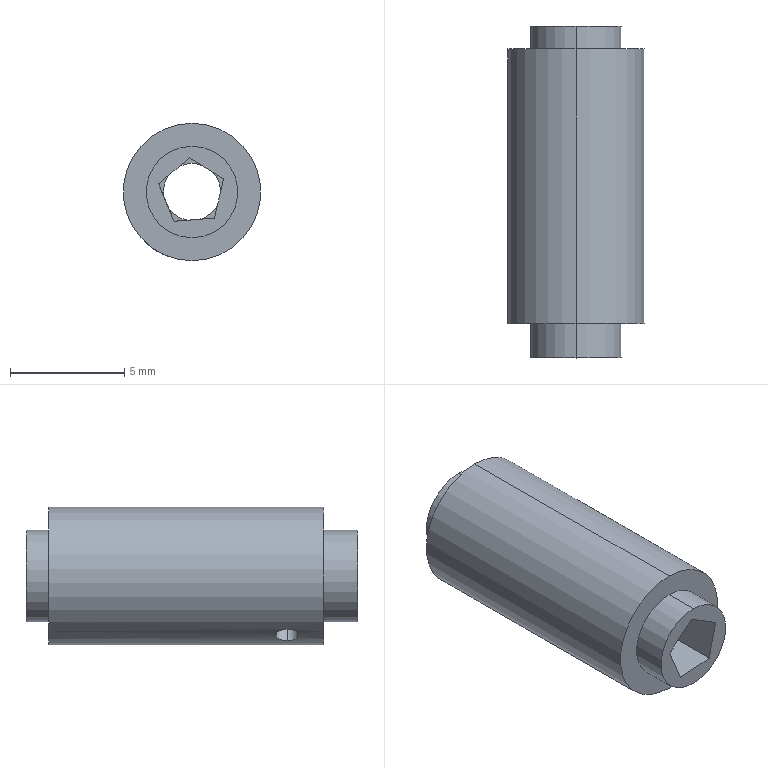Part | SolidWorks | features ICE 6, Extrusion 1 | 1 solid | 27 faces | box 6 x 14.5 x 6 mm | volume 290.19 mm3 | plane 15 | cylinder 12 | commonest cylinder face diameters 4 x4 1 x2 2.5 x2 3 x2 6 x2
STEP:
#1=CARTESIAN_POINT('',(-1.9,1.589,-2.322));
#2=VERTEX_POINT('',#1);
#3=CARTESIAN_POINT('',(-1.031,1.589,-2.817));
#4=VERTEX_POINT('',#3);
#5=CARTESIAN_POINT('',(-1.9,1.589,-2.322));
#6=CARTESIAN_POINT('',(-1.9,1.459,-2.322));
#7=CARTESIAN_POINT('',(-1.858,1.328,-2.357));
#8=CARTESIAN_POINT('',(-1.709,1.143,-2.467));
#9=CARTESIAN_POINT('',(-1.602,1.089,-2.54));
#10=CARTESIAN_POINT('',(-1.372,1.089,-2.671));
#11=CARTESIAN_POINT('',(-1.255,1.144,-2.727));
#12=CARTESIAN_POINT('',(-1.084,1.328,-2.799));
#13=CARTESIAN_POINT('',(-1.031,1.457,-2.817));
#14=CARTESIAN_POINT('',(-1.031,1.589,-2.817));
#15=B_SPLINE_CURVE_WITH_KNOTS('',3,(#5,#6,#7,#8,#9,#10,#11,#12,#13,#14),.UNSPECIFIED.,.F.,.F.,(4,2,2,2,4),(0.001566,0.001958,0.002349,0.002741,0.003132),.UNSPECIFIED.);
#16=EDGE_CURVE('',#2,#4,#15,.T.);
#17=ORIENTED_EDGE('',*,*,#16,.F.);
#18=CARTESIAN_POINT('',(-0.9761,1.589,-0.8146));
#19=VERTEX_POINT('',#18);
#20=CARTESIAN_POINT('',(-2.503,1.589,-3.306));
#21=DIRECTION('',(0.5226,0.,0.8526));
#22=VECTOR('',#21,1000.);
#23=LINE('',#20,#22);
#24=EDGE_CURVE('',#2,#19,#23,.T.);
#25=ORIENTED_EDGE('',*,*,#24,.T.);
#26=CARTESIAN_POINT('',(-0.7839,1.098,-1.279));
#27=VERTEX_POINT('',#26);
#28=CARTESIAN_POINT('',(-0.9761,1.589,-0.8146));
#29=CARTESIAN_POINT('',(-0.9761,1.338,-0.8146));
#30=CARTESIAN_POINT('',(-0.9005,1.145,-0.9973));
#31=CARTESIAN_POINT('',(-0.7839,1.098,-1.279));
#32=(BOUNDED_CURVE()B_SPLINE_CURVE(3,(#28,#29,#30,#31),.UNSPECIFIED.,.F.,.F.)B_SPLINE_CURVE_WITH_KNOTS((4,4),(3.142,4.524),.UNSPECIFIED.)CURVE()GEOMETRIC_REPRESENTATION_ITEM()RATIONAL_B_SPLINE_CURVE((1.,0.8469,0.8469,1.))REPRESENTATION_ITEM(''));
#33=EDGE_CURVE('',#19,#27,#32,.T.);
#34=ORIENTED_EDGE('',*,*,#33,.T.);
#35=CARTESIAN_POINT('',(-0.05259,1.589,-1.221));
#36=VERTEX_POINT('',#35);
#37=CARTESIAN_POINT('',(-0.7839,1.098,-1.279));
#38=CARTESIAN_POINT('',(-0.374,1.035,-1.247));
#39=CARTESIAN_POINT('',(-0.05259,1.251,-1.221));
#40=CARTESIAN_POINT('',(-0.05259,1.589,-1.221));
#41=(BOUNDED_CURVE()B_SPLINE_CURVE(3,(#37,#38,#39,#40),.UNSPECIFIED.,.F.,.F.)B_SPLINE_CURVE_WITH_KNOTS((4,4),(1.383,3.142),.UNSPECIFIED.)CURVE()GEOMETRIC_REPRESENTATION_ITEM()RATIONAL_B_SPLINE_CURVE((1.,0.7584,0.7584,1.))REPRESENTATION_ITEM(''));
#42=EDGE_CURVE('',#27,#36,#41,.T.);
#43=ORIENTED_EDGE('',*,*,#42,.T.);
#44=CARTESIAN_POINT('',(-1.651,1.589,-3.829));
#45=DIRECTION('',(0.5226,0.,0.8526));
#46=VECTOR('',#45,1000.);
#47=LINE('',#44,#46);
#48=EDGE_CURVE('',#4,#36,#47,.T.);
#49=ORIENTED_EDGE('',*,*,#48,.F.);
#50=EDGE_LOOP('',(#17,#25,#34,#43,#49));
#51=FACE_OUTER_BOUND('',#50,.T.);
#52=CARTESIAN_POINT('',(-2.077,1.589,-3.567));
#53=DIRECTION('',(0.5226,0.,0.8526));
#54=DIRECTION('',(0.8526,0.,-0.5226));
#55=AXIS2_PLACEMENT_3D('',#52,#53,#54);
#56=CYLINDRICAL_SURFACE('',#55,0.5);
#57=ADVANCED_FACE('',(#51),#56,.F.);
#58=CARTESIAN_POINT('',(0.,4.5,-1.5));
#59=VERTEX_POINT('',#58);
#60=CARTESIAN_POINT('',(-0.7839,4.5,-1.279));
#61=VERTEX_POINT('',#60);
#62=CARTESIAN_POINT('',(0.,4.5,0.));
#63=DIRECTION('',(0.,1.,0.));
#64=DIRECTION('',(0.,0.,1.));
#65=AXIS2_PLACEMENT_3D('',#62,#63,#64);
#66=CIRCLE('',#65,1.5);
#67=EDGE_CURVE('',#59,#61,#66,.T.);
#68=ORIENTED_EDGE('',*,*,#67,.F.);
#69=CARTESIAN_POINT('',(0.,7.,-1.5));
#70=VERTEX_POINT('',#69);
#71=CARTESIAN_POINT('',(0.,4.5,-1.5));
#72=DIRECTION('',(0.,1.,0.));
#73=VECTOR('',#72,1000.);
#74=LINE('',#71,#73);
#75=EDGE_CURVE('',#59,#70,#74,.T.);
#76=ORIENTED_EDGE('',*,*,#75,.T.);
#77=CARTESIAN_POINT('',(0.,7.,1.5));
#78=VERTEX_POINT('',#77);
#79=CARTESIAN_POINT('',(0.,7.,0.));
#80=DIRECTION('',(0.,1.,0.));
#81=DIRECTION('',(0.,0.,1.));
#82=AXIS2_PLACEMENT_3D('',#79,#80,#81);
#83=CIRCLE('',#82,1.5);
#84=EDGE_CURVE('',#70,#78,#83,.T.);
#85=ORIENTED_EDGE('',*,*,#84,.T.);
#86=CARTESIAN_POINT('',(0.,4.5,1.5));
#87=VERTEX_POINT('',#86);
#88=CARTESIAN_POINT('',(0.,4.5,1.5));
#89=DIRECTION('',(0.,1.,0.));
#90=VECTOR('',#89,1000.);
#91=LINE('',#88,#90);
#92=EDGE_CURVE('',#87,#78,#91,.T.);
#93=ORIENTED_EDGE('',*,*,#92,.F.);
#94=CARTESIAN_POINT('',(-0.1176,4.5,1.495));
#95=VERTEX_POINT('',#94);
#96=CARTESIAN_POINT('',(0.,4.5,0.));
#97=DIRECTION('',(0.,1.,0.));
#98=DIRECTION('',(0.,0.,1.));
#99=AXIS2_PLACEMENT_3D('',#96,#97,#98);
#100=CIRCLE('',#99,1.5);
#101=EDGE_CURVE('',#95,#87,#100,.T.);
#102=ORIENTED_EDGE('',*,*,#101,.F.);
#103=CARTESIAN_POINT('',(-1.459,4.5,0.3503));
#104=VERTEX_POINT('',#103);
#105=CARTESIAN_POINT('',(0.,4.5,0.));
#106=DIRECTION('',(0.,1.,0.));
#107=DIRECTION('',(0.,0.,1.));
#108=AXIS2_PLACEMENT_3D('',#105,#106,#107);
#109=CIRCLE('',#108,1.5);
#110=EDGE_CURVE('',#104,#95,#109,.T.);
#111=ORIENTED_EDGE('',*,*,#110,.F.);
#112=CARTESIAN_POINT('',(0.,4.5,0.));
#113=DIRECTION('',(0.,1.,0.));
#114=DIRECTION('',(0.,0.,1.));
#115=AXIS2_PLACEMENT_3D('',#112,#113,#114);
#116=CIRCLE('',#115,1.5);
#117=EDGE_CURVE('',#61,#104,#116,.T.);
#118=ORIENTED_EDGE('',*,*,#117,.F.);
#119=EDGE_LOOP('',(#68,#76,#85,#93,#102,#111,#118));
#120=FACE_OUTER_BOUND('',#119,.T.);
#121=CARTESIAN_POINT('',(0.,4.5,0.));
#122=DIRECTION('',(0.,1.,0.));
#123=DIRECTION('',(0.,0.,1.));
#124=AXIS2_PLACEMENT_3D('',#121,#122,#123);
#125=CYLINDRICAL_SURFACE('',#124,1.5);
#126=ADVANCED_FACE('',(#120),#125,.F.);
#127=CARTESIAN_POINT('',(0.,7.,-1.25));
#128=VERTEX_POINT('',#127);
#129=CARTESIAN_POINT('',(0.,7.,1.25));
#130=VERTEX_POINT('',#129);
#131=CARTESIAN_POINT('',(0.,7.,0.));
#132=DIRECTION('',(0.,1.,0.));
#133=DIRECTION('',(0.,0.,1.));
#134=AXIS2_PLACEMENT_3D('',#131,#132,#133);
#135=CIRCLE('',#134,1.25);
#136=EDGE_CURVE('',#128,#130,#135,.T.);
#137=ORIENTED_EDGE('',*,*,#136,.F.);
#138=CARTESIAN_POINT('',(0.,13.,-1.25));
#139=VERTEX_POINT('',#138);
#140=CARTESIAN_POINT('',(0.,7.,-1.25));
#141=DIRECTION('',(0.,1.,0.));
#142=VECTOR('',#141,1000.);
#143=LINE('',#140,#142);
#144=EDGE_CURVE('',#128,#139,#143,.T.);
#145=ORIENTED_EDGE('',*,*,#144,.T.);
#146=CARTESIAN_POINT('',(0.,13.,1.25));
#147=VERTEX_POINT('',#146);
#148=CARTESIAN_POINT('',(0.,13.,0.));
#149=DIRECTION('',(0.,1.,0.));
#150=DIRECTION('',(0.,0.,1.));
#151=AXIS2_PLACEMENT_3D('',#148,#149,#150);
#152=CIRCLE('',#151,1.25);
#153=EDGE_CURVE('',#139,#147,#152,.T.);
#154=ORIENTED_EDGE('',*,*,#153,.T.);
#155=CARTESIAN_POINT('',(0.,7.,1.25));
#156=DIRECTION('',(0.,1.,0.));
#157=VECTOR('',#156,1000.);
#158=LINE('',#155,#157);
#159=EDGE_CURVE('',#130,#147,#158,.T.);
#160=ORIENTED_EDGE('',*,*,#159,.F.);
#161=EDGE_LOOP('',(#137,#145,#154,#160));
#162=FACE_OUTER_BOUND('',#161,.T.);
#163=CARTESIAN_POINT('',(0.,7.,0.));
#164=DIRECTION('',(0.,1.,0.));
#165=DIRECTION('',(0.,0.,1.));
#166=AXIS2_PLACEMENT_3D('',#163,#164,#165);
#167=CYLINDRICAL_SURFACE('',#166,1.25);
#168=ADVANCED_FACE('',(#162),#167,.F.);
#169=CARTESIAN_POINT('',(0.,-1.5,-2.));
#170=VERTEX_POINT('',#169);
#171=CARTESIAN_POINT('',(0.,-1.5,2.));
#172=VERTEX_POINT('',#171);
#173=CARTESIAN_POINT('',(0.,-1.5,0.));
#174=DIRECTION('',(0.,-1.,0.));
#175=DIRECTION('',(0.,0.,-1.));
#176=AXIS2_PLACEMENT_3D('',#173,#174,#175);
#177=CIRCLE('',#176,2.);
#178=EDGE_CURVE('',#170,#172,#177,.T.);
#179=ORIENTED_EDGE('',*,*,#178,.F.);
#180=CARTESIAN_POINT('',(0.,0.,-2.));
#181=VERTEX_POINT('',#180);
#182=CARTESIAN_POINT('',(0.,-1.5,-2.));
#183=DIRECTION('',(0.,1.,0.));
#184=VECTOR('',#183,1000.);
#185=LINE('',#182,#184);
#186=EDGE_CURVE('',#170,#181,#185,.T.);
#187=ORIENTED_EDGE('',*,*,#186,.T.);
#188=CARTESIAN_POINT('',(0.,0.,2.));
#189=VERTEX_POINT('',#188);
#190=CARTESIAN_POINT('',(0.,0.,0.));
#191=DIRECTION('',(0.,-1.,0.));
#192=DIRECTION('',(0.,0.,-1.));
#193=AXIS2_PLACEMENT_3D('',#190,#191,#192);
#194=CIRCLE('',#193,2.);
#195=EDGE_CURVE('',#181,#189,#194,.T.);
#196=ORIENTED_EDGE('',*,*,#195,.T.);
#197=CARTESIAN_POINT('',(0.,-1.5,2.));
#198=DIRECTION('',(0.,1.,0.));
#199=VECTOR('',#198,1000.);
#200=LINE('',#197,#199);
#201=EDGE_CURVE('',#172,#189,#200,.T.);
#202=ORIENTED_EDGE('',*,*,#201,.F.);
#203=EDGE_LOOP('',(#179,#187,#196,#202));
#204=FACE_OUTER_BOUND('',#203,.T.);
#205=CARTESIAN_POINT('',(0.,-1.5,0.));
#206=DIRECTION('',(0.,1.,0.));
#207=DIRECTION('',(0.,0.,1.));
#208=AXIS2_PLACEMENT_3D('',#205,#206,#207);
#209=CYLINDRICAL_SURFACE('',#208,2.);
#210=ADVANCED_FACE('',(#204),#209,.T.);
#211=CARTESIAN_POINT('',(0.,13.,2.));
#212=VERTEX_POINT('',#211);
#213=CARTESIAN_POINT('',(0.,13.,-2.));
#214=VERTEX_POINT('',#213);
#215=CARTESIAN_POINT('',(0.,13.,0.));
#216=DIRECTION('',(0.,1.,0.));
#217=DIRECTION('',(0.,0.,1.));
#218=AXIS2_PLACEMENT_3D('',#215,#216,#217);
#219=CIRCLE('',#218,2.);
#220=EDGE_CURVE('',#212,#214,#219,.T.);
#221=ORIENTED_EDGE('',*,*,#220,.F.);
#222=CARTESIAN_POINT('',(0.,12.,2.));
#223=VERTEX_POINT('',#222);
#224=CARTESIAN_POINT('',(0.,13.,2.));
#225=DIRECTION('',(0.,-1.,0.));
#226=VECTOR('',#225,1000.);
#227=LINE('',#224,#226);
#228=EDGE_CURVE('',#212,#223,#227,.T.);
#229=ORIENTED_EDGE('',*,*,#228,.T.);
#230=CARTESIAN_POINT('',(0.,12.,-2.));
#231=VERTEX_POINT('',#230);
#232=CARTESIAN_POINT('',(0.,12.,0.));
#233=DIRECTION('',(0.,1.,0.));
#234=DIRECTION('',(0.,0.,1.));
#235=AXIS2_PLACEMENT_3D('',#232,#233,#234);
#236=CIRCLE('',#235,2.);
#237=EDGE_CURVE('',#223,#231,#236,.T.);
#238=ORIENTED_EDGE('',*,*,#237,.T.);
#239=CARTESIAN_POINT('',(0.,13.,-2.));
#240=DIRECTION('',(0.,-1.,0.));
#241=VECTOR('',#240,1000.);
#242=LINE('',#239,#241);
#243=EDGE_CURVE('',#214,#231,#242,.T.);
#244=ORIENTED_EDGE('',*,*,#243,.F.);
#245=EDGE_LOOP('',(#221,#229,#238,#244));
#246=FACE_OUTER_BOUND('',#245,.T.);
#247=CARTESIAN_POINT('',(0.,13.,0.));
#248=DIRECTION('',(0.,-1.,0.));
#249=DIRECTION('',(0.,0.,-1.));
#250=AXIS2_PLACEMENT_3D('',#247,#248,#249);
#251=CYLINDRICAL_SURFACE('',#250,2.);
#252=ADVANCED_FACE('',(#246),#251,.T.);
#253=CARTESIAN_POINT('',(0.,12.,3.));
#254=VERTEX_POINT('',#253);
#255=CARTESIAN_POINT('',(0.,12.,-3.));
#256=VERTEX_POINT('',#255);
#257=CARTESIAN_POINT('',(0.,12.,0.));
#258=DIRECTION('',(0.,1.,0.));
#259=DIRECTION('',(0.,0.,1.));
#260=AXIS2_PLACEMENT_3D('',#257,#258,#259);
#261=CIRCLE('',#260,3.);
#262=EDGE_CURVE('',#254,#256,#261,.T.);
#263=ORIENTED_EDGE('',*,*,#262,.F.);
#264=CARTESIAN_POINT('',(0.,0.,3.));
#265=VERTEX_POINT('',#264);
#266=CARTESIAN_POINT('',(0.,12.,3.));
#267=DIRECTION('',(0.,-1.,0.));
#268=VECTOR('',#267,1000.);
#269=LINE('',#266,#268);
#270=EDGE_CURVE('',#254,#265,#269,.T.);
#271=ORIENTED_EDGE('',*,*,#270,.T.);
#272=CARTESIAN_POINT('',(0.,0.,-3.));
#273=VERTEX_POINT('',#272);
#274=CARTESIAN_POINT('',(0.,0.,0.));
#275=DIRECTION('',(0.,1.,0.));
#276=DIRECTION('',(0.,0.,1.));
#277=AXIS2_PLACEMENT_3D('',#274,#275,#276);
#278=CIRCLE('',#277,3.);
#279=EDGE_CURVE('',#265,#273,#278,.T.);
#280=ORIENTED_EDGE('',*,*,#279,.T.);
#281=CARTESIAN_POINT('',(0.,12.,-3.));
#282=DIRECTION('',(0.,-1.,0.));
#283=VECTOR('',#282,1000.);
#284=LINE('',#281,#283);
#285=EDGE_CURVE('',#256,#273,#284,.T.);
#286=ORIENTED_EDGE('',*,*,#285,.F.);
#287=EDGE_LOOP('',(#263,#271,#280,#286));
#288=FACE_OUTER_BOUND('',#287,.T.);
#289=CARTESIAN_POINT('',(0.,12.,0.));
#290=DIRECTION('',(0.,-1.,0.));
#291=DIRECTION('',(0.,0.,-1.));
#292=AXIS2_PLACEMENT_3D('',#289,#290,#291);
#293=CYLINDRICAL_SURFACE('',#292,3.);
#294=ADVANCED_FACE('',(#288),#293,.T.);
#295=ORIENTED_EDGE('',*,*,#270,.F.);
#296=CARTESIAN_POINT('',(0.,12.,0.));
#297=DIRECTION('',(0.,1.,0.));
#298=DIRECTION('',(0.,0.,1.));
#299=AXIS2_PLACEMENT_3D('',#296,#297,#298);
#300=CIRCLE('',#299,3.);
#301=EDGE_CURVE('',#256,#254,#300,.T.);
#302=ORIENTED_EDGE('',*,*,#301,.F.);
#303=ORIENTED_EDGE('',*,*,#285,.T.);
#304=CARTESIAN_POINT('',(0.,0.,0.));
#305=DIRECTION('',(0.,1.,0.));
#306=DIRECTION('',(0.,0.,1.));
#307=AXIS2_PLACEMENT_3D('',#304,#305,#306);
#308=CIRCLE('',#307,3.);
#309=EDGE_CURVE('',#273,#265,#308,.T.);
#310=ORIENTED_EDGE('',*,*,#309,.T.);
#311=EDGE_LOOP('',(#295,#302,#303,#310));
#312=FACE_OUTER_BOUND('',#311,.T.);
#313=CARTESIAN_POINT('',(-1.031,1.589,-2.817));
#314=CARTESIAN_POINT('',(-1.031,1.722,-2.817));
#315=CARTESIAN_POINT('',(-1.083,1.851,-2.799));
#316=CARTESIAN_POINT('',(-1.255,2.035,-2.727));
#317=CARTESIAN_POINT('',(-1.373,2.089,-2.671));
#318=CARTESIAN_POINT('',(-1.6,2.09,-2.541));
#319=CARTESIAN_POINT('',(-1.708,2.036,-2.468));
#320=CARTESIAN_POINT('',(-1.859,1.85,-2.357));
#321=CARTESIAN_POINT('',(-1.9,1.72,-2.322));
#322=CARTESIAN_POINT('',(-1.9,1.589,-2.322));
#323=B_SPLINE_CURVE_WITH_KNOTS('',3,(#313,#314,#315,#316,#317,#318,#319,#320,#321,#322),.UNSPECIFIED.,.F.,.F.,(4,2,2,2,4),(0.,0.0003916,0.0007832,0.001175,0.001566),.UNSPECIFIED.);
#324=EDGE_CURVE('',#4,#2,#323,.T.);
#325=ORIENTED_EDGE('',*,*,#324,.T.);
#326=ORIENTED_EDGE('',*,*,#16,.T.);
#327=EDGE_LOOP('',(#325,#326));
#328=FACE_BOUND('',#327,.T.);
#329=CARTESIAN_POINT('',(0.,12.,0.));
#330=DIRECTION('',(0.,-1.,0.));
#331=DIRECTION('',(0.,0.,-1.));
#332=AXIS2_PLACEMENT_3D('',#329,#330,#331);
#333=CYLINDRICAL_SURFACE('',#332,3.);
#334=ADVANCED_FACE('',(#312,#328),#333,.T.);
#335=ORIENTED_EDGE('',*,*,#42,.F.);
#336=CARTESIAN_POINT('',(-0.7839,-1.5,-1.279));
#337=VERTEX_POINT('',#336);
#338=CARTESIAN_POINT('',(-0.7839,4.5,-1.279));
#339=DIRECTION('',(0.,-1.,0.));
#340=VECTOR('',#339,1000.);
#341=LINE('',#338,#340);
#342=EDGE_CURVE('',#27,#337,#341,.T.);
#343=ORIENTED_EDGE('',*,*,#342,.T.);
#344=CARTESIAN_POINT('',(0.9741,-1.5,-1.141));
#345=VERTEX_POINT('',#344);
#346=CARTESIAN_POINT('',(-0.7839,-1.5,-1.279));
#347=DIRECTION('',(0.9969,0.,0.07838));
#348=VECTOR('',#347,1000.);
#349=LINE('',#346,#348);
#350=EDGE_CURVE('',#337,#345,#349,.T.);
#351=ORIENTED_EDGE('',*,*,#350,.T.);
#352=CARTESIAN_POINT('',(0.9741,4.5,-1.141));
#353=VERTEX_POINT('',#352);
#354=CARTESIAN_POINT('',(0.9741,4.5,-1.141));
#355=DIRECTION('',(0.,-1.,0.));
#356=VECTOR('',#355,1000.);
#357=LINE('',#354,#356);
#358=EDGE_CURVE('',#353,#345,#357,.T.);
#359=ORIENTED_EDGE('',*,*,#358,.F.);
#360=CARTESIAN_POINT('',(-0.7839,4.5,-1.279));
#361=DIRECTION('',(0.9969,0.,0.07838));
#362=VECTOR('',#361,1000.);
#363=LINE('',#360,#362);
#364=EDGE_CURVE('',#61,#353,#363,.T.);
#365=ORIENTED_EDGE('',*,*,#364,.F.);
#366=CARTESIAN_POINT('',(-0.7839,2.081,-1.279));
#367=VERTEX_POINT('',#366);
#368=CARTESIAN_POINT('',(-0.7839,4.5,-1.279));
#369=DIRECTION('',(0.,-1.,0.));
#370=VECTOR('',#369,1000.);
#371=LINE('',#368,#370);
#372=EDGE_CURVE('',#61,#367,#371,.T.);
#373=ORIENTED_EDGE('',*,*,#372,.T.);
#374=CARTESIAN_POINT('',(-0.05259,1.589,-1.221));
#375=CARTESIAN_POINT('',(-0.05259,1.928,-1.221));
#376=CARTESIAN_POINT('',(-0.374,2.144,-1.247));
#377=CARTESIAN_POINT('',(-0.7839,2.081,-1.279));
#378=(BOUNDED_CURVE()B_SPLINE_CURVE(3,(#374,#375,#376,#377),.UNSPECIFIED.,.F.,.F.)B_SPLINE_CURVE_WITH_KNOTS((4,4),(3.142,4.9),.UNSPECIFIED.)CURVE()GEOMETRIC_REPRESENTATION_ITEM()RATIONAL_B_SPLINE_CURVE((1.,0.7584,0.7584,1.))REPRESENTATION_ITEM(''));
#379=EDGE_CURVE('',#36,#367,#378,.T.);
#380=ORIENTED_EDGE('',*,*,#379,.F.);
#381=EDGE_LOOP('',(#335,#343,#351,#359,#365,#373,#380));
#382=FACE_OUTER_BOUND('',#381,.T.);
#383=CARTESIAN_POINT('',(-0.7839,4.5,-1.279));
#384=DIRECTION('',(0.07838,0.,-0.9969));
#385=DIRECTION('',(-0.9969,0.,-0.07838));
#386=AXIS2_PLACEMENT_3D('',#383,#384,#385);
#387=PLANE('',#386);
#388=ADVANCED_FACE('',(#382),#387,.F.);
#389=CARTESIAN_POINT('',(-0.7839,2.081,-1.279));
#390=CARTESIAN_POINT('',(-0.9005,2.034,-0.9973));
#391=CARTESIAN_POINT('',(-0.9761,1.84,-0.8146));
#392=CARTESIAN_POINT('',(-0.9761,1.589,-0.8146));
#393=(BOUNDED_CURVE()B_SPLINE_CURVE(3,(#389,#390,#391,#392),.UNSPECIFIED.,.F.,.T.)B_SPLINE_CURVE_WITH_KNOTS((4,4),(1.759,3.142),.UNSPECIFIED.)CURVE()GEOMETRIC_REPRESENTATION_ITEM()RATIONAL_B_SPLINE_CURVE((1.,0.8469,0.8469,1.))REPRESENTATION_ITEM(''));
#394=EDGE_CURVE('',#367,#19,#393,.T.);
#395=ORIENTED_EDGE('',*,*,#394,.F.);
#396=ORIENTED_EDGE('',*,*,#372,.F.);
#397=CARTESIAN_POINT('',(-1.459,4.5,0.3503));
#398=DIRECTION('',(0.3826,0.,-0.9239));
#399=VECTOR('',#398,1000.);
#400=LINE('',#397,#399);
#401=EDGE_CURVE('',#104,#61,#400,.T.);
#402=ORIENTED_EDGE('',*,*,#401,.F.);
#403=CARTESIAN_POINT('',(-1.459,-1.5,0.3503));
#404=VERTEX_POINT('',#403);
#405=CARTESIAN_POINT('',(-1.459,4.5,0.3503));
#406=DIRECTION('',(0.,-1.,0.));
#407=VECTOR('',#406,1000.);
#408=LINE('',#405,#407);
#409=EDGE_CURVE('',#104,#404,#408,.T.);
#410=ORIENTED_EDGE('',*,*,#409,.T.);
#411=CARTESIAN_POINT('',(-1.459,-1.5,0.3503));
#412=DIRECTION('',(0.3826,0.,-0.9239));
#413=VECTOR('',#412,1000.);
#414=LINE('',#411,#413);
#415=EDGE_CURVE('',#404,#337,#414,.T.);
#416=ORIENTED_EDGE('',*,*,#415,.T.);
#417=ORIENTED_EDGE('',*,*,#342,.F.);
#418=ORIENTED_EDGE('',*,*,#33,.F.);
#419=EDGE_LOOP('',(#395,#396,#402,#410,#416,#417,#418));
#420=FACE_OUTER_BOUND('',#419,.T.);
#421=CARTESIAN_POINT('',(-1.459,4.5,0.3503));
#422=DIRECTION('',(-0.9239,0.,-0.3826));
#423=DIRECTION('',(-0.3826,0.,0.9239));
#424=AXIS2_PLACEMENT_3D('',#421,#422,#423);
#425=PLANE('',#424);
#426=ADVANCED_FACE('',(#420),#425,.F.);
#427=CARTESIAN_POINT('',(0.,4.5,0.));
#428=DIRECTION('',(0.,1.,0.));
#429=DIRECTION('',(0.,0.,1.));
#430=AXIS2_PLACEMENT_3D('',#427,#428,#429);
#431=CIRCLE('',#430,1.5);
#432=EDGE_CURVE('',#353,#59,#431,.T.);
#433=ORIENTED_EDGE('',*,*,#432,.T.);
#434=ORIENTED_EDGE('',*,*,#67,.T.);
#435=ORIENTED_EDGE('',*,*,#364,.T.);
#436=EDGE_LOOP('',(#433,#434,#435));
#437=FACE_OUTER_BOUND('',#436,.T.);
#438=CARTESIAN_POINT('',(0.,4.5,0.));
#439=DIRECTION('',(0.,1.,0.));
#440=DIRECTION('',(0.,0.,1.));
#441=AXIS2_PLACEMENT_3D('',#438,#439,#440);
#442=PLANE('',#441);
#443=ADVANCED_FACE('',(#437),#442,.T.);
#444=ORIENTED_EDGE('',*,*,#117,.T.);
#445=ORIENTED_EDGE('',*,*,#401,.T.);
#446=EDGE_LOOP('',(#444,#445));
#447=FACE_OUTER_BOUND('',#446,.T.);
#448=CARTESIAN_POINT('',(0.,4.5,0.));
#449=DIRECTION('',(0.,1.,0.));
#450=DIRECTION('',(0.,0.,1.));
#451=AXIS2_PLACEMENT_3D('',#448,#449,#450);
#452=PLANE('',#451);
#453=ADVANCED_FACE('',(#447),#452,.T.);
#454=ORIENTED_EDGE('',*,*,#110,.T.);
#455=CARTESIAN_POINT('',(-0.1176,4.5,1.495));
#456=DIRECTION('',(-0.7605,0.,-0.6494));
#457=VECTOR('',#456,1000.);
#458=LINE('',#455,#457);
#459=EDGE_CURVE('',#95,#104,#458,.T.);
#460=ORIENTED_EDGE('',*,*,#459,.T.);
#461=EDGE_LOOP('',(#454,#460));
#462=FACE_OUTER_BOUND('',#461,.T.);
#463=CARTESIAN_POINT('',(0.,4.5,0.));
#464=DIRECTION('',(0.,1.,0.));
#465=DIRECTION('',(0.,0.,1.));
#466=AXIS2_PLACEMENT_3D('',#463,#464,#465);
#467=PLANE('',#466);
#468=ADVANCED_FACE('',(#462),#467,.T.);
#469=ORIENTED_EDGE('',*,*,#101,.T.);
#470=CARTESIAN_POINT('',(1.386,4.5,0.5739));
#471=VERTEX_POINT('',#470);
#472=CARTESIAN_POINT('',(0.,4.5,0.));
#473=DIRECTION('',(0.,1.,0.));
#474=DIRECTION('',(0.,0.,1.));
#475=AXIS2_PLACEMENT_3D('',#472,#473,#474);
#476=CIRCLE('',#475,1.5);
#477=EDGE_CURVE('',#87,#471,#476,.T.);
#478=ORIENTED_EDGE('',*,*,#477,.T.);
#479=CARTESIAN_POINT('',(1.386,4.5,0.5739));
#480=DIRECTION('',(-0.8526,0.,0.5226));
#481=VECTOR('',#480,1000.);
#482=LINE('',#479,#481);
#483=EDGE_CURVE('',#471,#95,#482,.T.);
#484=ORIENTED_EDGE('',*,*,#483,.T.);
#485=EDGE_LOOP('',(#469,#478,#484));
#486=FACE_OUTER_BOUND('',#485,.T.);
#487=CARTESIAN_POINT('',(0.,4.5,0.));
#488=DIRECTION('',(0.,1.,0.));
#489=DIRECTION('',(0.,0.,1.));
#490=AXIS2_PLACEMENT_3D('',#487,#488,#489);
#491=PLANE('',#490);
#492=ADVANCED_FACE('',(#486),#491,.T.);
#493=CARTESIAN_POINT('',(0.,4.5,0.));
#494=DIRECTION('',(0.,1.,0.));
#495=DIRECTION('',(0.,0.,1.));
#496=AXIS2_PLACEMENT_3D('',#493,#494,#495);
#497=CIRCLE('',#496,1.5);
#498=EDGE_CURVE('',#471,#353,#497,.T.);
#499=ORIENTED_EDGE('',*,*,#498,.T.);
#500=CARTESIAN_POINT('',(0.9741,4.5,-1.141));
#501=DIRECTION('',(0.2335,0.,0.9724));
#502=VECTOR('',#501,1000.);
#503=LINE('',#500,#502);
#504=EDGE_CURVE('',#353,#471,#503,.T.);
#505=ORIENTED_EDGE('',*,*,#504,.T.);
#506=EDGE_LOOP('',(#499,#505));
#507=FACE_OUTER_BOUND('',#506,.T.);
#508=CARTESIAN_POINT('',(0.,4.5,0.));
#509=DIRECTION('',(0.,1.,0.));
#510=DIRECTION('',(0.,0.,1.));
#511=AXIS2_PLACEMENT_3D('',#508,#509,#510);
#512=PLANE('',#511);
#513=ADVANCED_FACE('',(#507),#512,.T.);
#514=CARTESIAN_POINT('',(0.,12.,0.));
#515=DIRECTION('',(0.,1.,0.));
#516=DIRECTION('',(0.,0.,1.));
#517=AXIS2_PLACEMENT_3D('',#514,#515,#516);
#518=CIRCLE('',#517,2.);
#519=EDGE_CURVE('',#231,#223,#518,.T.);
#520=ORIENTED_EDGE('',*,*,#519,.F.);
#521=ORIENTED_EDGE('',*,*,#237,.F.);
#522=EDGE_LOOP('',(#520,#521));
#523=FACE_BOUND('',#522,.T.);
#524=ORIENTED_EDGE('',*,*,#301,.T.);
#525=ORIENTED_EDGE('',*,*,#262,.T.);
#526=EDGE_LOOP('',(#524,#525));
#527=FACE_OUTER_BOUND('',#526,.T.);
#528=CARTESIAN_POINT('',(0.,12.,0.));
#529=DIRECTION('',(0.,1.,0.));
#530=DIRECTION('',(0.,0.,1.));
#531=AXIS2_PLACEMENT_3D('',#528,#529,#530);
#532=PLANE('',#531);
#533=ADVANCED_FACE('',(#523,#527),#532,.T.);
#534=CARTESIAN_POINT('',(0.,0.,0.));
#535=DIRECTION('',(0.,-1.,0.));
#536=DIRECTION('',(0.,0.,-1.));
#537=AXIS2_PLACEMENT_3D('',#534,#535,#536);
#538=CIRCLE('',#537,2.);
#539=EDGE_CURVE('',#189,#181,#538,.T.);
#540=ORIENTED_EDGE('',*,*,#539,.F.);
#541=ORIENTED_EDGE('',*,*,#195,.F.);
#542=EDGE_LOOP('',(#540,#541));
#543=FACE_BOUND('',#542,.T.);
#544=ORIENTED_EDGE('',*,*,#309,.F.);
#545=ORIENTED_EDGE('',*,*,#279,.F.);
#546=EDGE_LOOP('',(#544,#545));
#547=FACE_OUTER_BOUND('',#546,.T.);
#548=CARTESIAN_POINT('',(0.,0.,0.));
#549=DIRECTION('',(0.,1.,0.));
#550=DIRECTION('',(0.,0.,1.));
#551=AXIS2_PLACEMENT_3D('',#548,#549,#550);
#552=PLANE('',#551);
#553=ADVANCED_FACE('',(#543,#547),#552,.F.);
#554=ORIENTED_EDGE('',*,*,#228,.F.);
#555=CARTESIAN_POINT('',(0.,13.,0.));
#556=DIRECTION('',(0.,1.,0.));
#557=DIRECTION('',(0.,0.,1.));
#558=AXIS2_PLACEMENT_3D('',#555,#556,#557);
#559=CIRCLE('',#558,2.);
#560=EDGE_CURVE('',#214,#212,#559,.T.);
#561=ORIENTED_EDGE('',*,*,#560,.F.);
#562=ORIENTED_EDGE('',*,*,#243,.T.);
#563=ORIENTED_EDGE('',*,*,#519,.T.);
#564=EDGE_LOOP('',(#554,#561,#562,#563));
#565=FACE_OUTER_BOUND('',#564,.T.);
#566=CARTESIAN_POINT('',(0.,13.,0.));
#567=DIRECTION('',(0.,-1.,0.));
#568=DIRECTION('',(0.,0.,-1.));
#569=AXIS2_PLACEMENT_3D('',#566,#567,#568);
#570=CYLINDRICAL_SURFACE('',#569,2.);
#571=ADVANCED_FACE('',(#565),#570,.T.);
#572=CARTESIAN_POINT('',(0.,13.,0.));
#573=DIRECTION('',(0.,1.,0.));
#574=DIRECTION('',(0.,0.,1.));
#575=AXIS2_PLACEMENT_3D('',#572,#573,#574);
#576=CIRCLE('',#575,1.25);
#577=EDGE_CURVE('',#147,#139,#576,.T.);
#578=ORIENTED_EDGE('',*,*,#577,.F.);
#579=ORIENTED_EDGE('',*,*,#153,.F.);
#580=EDGE_LOOP('',(#578,#579));
#581=FACE_BOUND('',#580,.T.);
#582=ORIENTED_EDGE('',*,*,#560,.T.);
#583=ORIENTED_EDGE('',*,*,#220,.T.);
#584=EDGE_LOOP('',(#582,#583));
#585=FACE_OUTER_BOUND('',#584,.T.);
#586=CARTESIAN_POINT('',(0.,13.,0.));
#587=DIRECTION('',(0.,1.,0.));
#588=DIRECTION('',(0.,0.,1.));
#589=AXIS2_PLACEMENT_3D('',#586,#587,#588);
#590=PLANE('',#589);
#591=ADVANCED_FACE('',(#581,#585),#590,.T.);
#592=ORIENTED_EDGE('',*,*,#186,.F.);
#593=CARTESIAN_POINT('',(0.,-1.5,0.));
#594=DIRECTION('',(0.,-1.,0.));
#595=DIRECTION('',(0.,0.,-1.));
#596=AXIS2_PLACEMENT_3D('',#593,#594,#595);
#597=CIRCLE('',#596,2.);
#598=EDGE_CURVE('',#172,#170,#597,.T.);
#599=ORIENTED_EDGE('',*,*,#598,.F.);
#600=ORIENTED_EDGE('',*,*,#201,.T.);
#601=ORIENTED_EDGE('',*,*,#539,.T.);
#602=EDGE_LOOP('',(#592,#599,#600,#601));
#603=FACE_OUTER_BOUND('',#602,.T.);
#604=CARTESIAN_POINT('',(0.,-1.5,0.));
#605=DIRECTION('',(0.,1.,0.));
#606=DIRECTION('',(0.,0.,1.));
#607=AXIS2_PLACEMENT_3D('',#604,#605,#606);
#608=CYLINDRICAL_SURFACE('',#607,2.);
#609=ADVANCED_FACE('',(#603),#608,.T.);
#610=ORIENTED_EDGE('',*,*,#350,.F.);
#611=ORIENTED_EDGE('',*,*,#415,.F.);
#612=CARTESIAN_POINT('',(-0.1176,-1.5,1.495));
#613=VERTEX_POINT('',#612);
#614=CARTESIAN_POINT('',(-0.1176,-1.5,1.495));
#615=DIRECTION('',(-0.7605,0.,-0.6494));
#616=VECTOR('',#615,1000.);
#617=LINE('',#614,#616);
#618=EDGE_CURVE('',#613,#404,#617,.T.);
#619=ORIENTED_EDGE('',*,*,#618,.F.);
#620=CARTESIAN_POINT('',(1.386,-1.5,0.5739));
#621=VERTEX_POINT('',#620);
#622=CARTESIAN_POINT('',(1.386,-1.5,0.5739));
#623=DIRECTION('',(-0.8526,0.,0.5226));
#624=VECTOR('',#623,1000.);
#625=LINE('',#622,#624);
#626=EDGE_CURVE('',#621,#613,#625,.T.);
#627=ORIENTED_EDGE('',*,*,#626,.F.);
#628=CARTESIAN_POINT('',(0.9741,-1.5,-1.141));
#629=DIRECTION('',(0.2335,0.,0.9724));
#630=VECTOR('',#629,1000.);
#631=LINE('',#628,#630);
#632=EDGE_CURVE('',#345,#621,#631,.T.);
#633=ORIENTED_EDGE('',*,*,#632,.F.);
#634=EDGE_LOOP('',(#610,#611,#619,#627,#633));
#635=FACE_BOUND('',#634,.T.);
#636=ORIENTED_EDGE('',*,*,#598,.T.);
#637=ORIENTED_EDGE('',*,*,#178,.T.);
#638=EDGE_LOOP('',(#636,#637));
#639=FACE_OUTER_BOUND('',#638,.T.);
#640=CARTESIAN_POINT('',(0.,-1.5,0.));
#641=DIRECTION('',(0.,-1.,0.));
#642=DIRECTION('',(0.,0.,-1.));
#643=AXIS2_PLACEMENT_3D('',#640,#641,#642);
#644=PLANE('',#643);
#645=ADVANCED_FACE('',(#635,#639),#644,.T.);
#646=ORIENTED_EDGE('',*,*,#144,.F.);
#647=CARTESIAN_POINT('',(0.,7.,0.));
#648=DIRECTION('',(0.,1.,0.));
#649=DIRECTION('',(0.,0.,1.));
#650=AXIS2_PLACEMENT_3D('',#647,#648,#649);
#651=CIRCLE('',#650,1.25);
#652=EDGE_CURVE('',#130,#128,#651,.T.);
#653=ORIENTED_EDGE('',*,*,#652,.F.);
#654=ORIENTED_EDGE('',*,*,#159,.T.);
#655=ORIENTED_EDGE('',*,*,#577,.T.);
#656=EDGE_LOOP('',(#646,#653,#654,#655));
#657=FACE_OUTER_BOUND('',#656,.T.);
#658=CARTESIAN_POINT('',(0.,7.,0.));
#659=DIRECTION('',(0.,1.,0.));
#660=DIRECTION('',(0.,0.,1.));
#661=AXIS2_PLACEMENT_3D('',#658,#659,#660);
#662=CYLINDRICAL_SURFACE('',#661,1.25);
#663=ADVANCED_FACE('',(#657),#662,.F.);
#664=ORIENTED_EDGE('',*,*,#75,.F.);
#665=ORIENTED_EDGE('',*,*,#432,.F.);
#666=ORIENTED_EDGE('',*,*,#498,.F.);
#667=ORIENTED_EDGE('',*,*,#477,.F.);
#668=ORIENTED_EDGE('',*,*,#92,.T.);
#669=CARTESIAN_POINT('',(0.,7.,0.));
#670=DIRECTION('',(0.,1.,0.));
#671=DIRECTION('',(0.,0.,1.));
#672=AXIS2_PLACEMENT_3D('',#669,#670,#671);
#673=CIRCLE('',#672,1.5);
#674=EDGE_CURVE('',#78,#70,#673,.T.);
#675=ORIENTED_EDGE('',*,*,#674,.T.);
#676=EDGE_LOOP('',(#664,#665,#666,#667,#668,#675));
#677=FACE_OUTER_BOUND('',#676,.T.);
#678=CARTESIAN_POINT('',(0.,4.5,0.));
#679=DIRECTION('',(0.,1.,0.));
#680=DIRECTION('',(0.,0.,1.));
#681=AXIS2_PLACEMENT_3D('',#678,#679,#680);
#682=CYLINDRICAL_SURFACE('',#681,1.5);
#683=ADVANCED_FACE('',(#677),#682,.F.);
#684=ORIENTED_EDGE('',*,*,#652,.T.);
#685=ORIENTED_EDGE('',*,*,#136,.T.);
#686=EDGE_LOOP('',(#684,#685));
#687=FACE_BOUND('',#686,.T.);
#688=ORIENTED_EDGE('',*,*,#674,.F.);
#689=ORIENTED_EDGE('',*,*,#84,.F.);
#690=EDGE_LOOP('',(#688,#689));
#691=FACE_OUTER_BOUND('',#690,.T.);
#692=CARTESIAN_POINT('',(0.,7.,0.));
#693=DIRECTION('',(0.,1.,0.));
#694=DIRECTION('',(0.,0.,1.));
#695=AXIS2_PLACEMENT_3D('',#692,#693,#694);
#696=PLANE('',#695);
#697=ADVANCED_FACE('',(#687,#691),#696,.F.);
#698=ORIENTED_EDGE('',*,*,#618,.T.);
#699=ORIENTED_EDGE('',*,*,#409,.F.);
#700=ORIENTED_EDGE('',*,*,#459,.F.);
#701=CARTESIAN_POINT('',(-0.1176,4.5,1.495));
#702=DIRECTION('',(0.,-1.,0.));
#703=VECTOR('',#702,1000.);
#704=LINE('',#701,#703);
#705=EDGE_CURVE('',#95,#613,#704,.T.);
#706=ORIENTED_EDGE('',*,*,#705,.T.);
#707=EDGE_LOOP('',(#698,#699,#700,#706));
#708=FACE_OUTER_BOUND('',#707,.T.);
#709=CARTESIAN_POINT('',(-0.1176,4.5,1.495));
#710=DIRECTION('',(-0.6494,0.,0.7605));
#711=DIRECTION('',(0.7605,0.,0.6494));
#712=AXIS2_PLACEMENT_3D('',#709,#710,#711);
#713=PLANE('',#712);
#714=ADVANCED_FACE('',(#708),#713,.F.);
#715=ORIENTED_EDGE('',*,*,#626,.T.);
#716=ORIENTED_EDGE('',*,*,#705,.F.);
#717=ORIENTED_EDGE('',*,*,#483,.F.);
#718=CARTESIAN_POINT('',(1.386,4.5,0.5739));
#719=DIRECTION('',(0.,-1.,0.));
#720=VECTOR('',#719,1000.);
#721=LINE('',#718,#720);
#722=EDGE_CURVE('',#471,#621,#721,.T.);
#723=ORIENTED_EDGE('',*,*,#722,.T.);
#724=EDGE_LOOP('',(#715,#716,#717,#723));
#725=FACE_OUTER_BOUND('',#724,.T.);
#726=CARTESIAN_POINT('',(1.386,4.5,0.5739));
#727=DIRECTION('',(0.5226,0.,0.8526));
#728=DIRECTION('',(0.8526,0.,-0.5226));
#729=AXIS2_PLACEMENT_3D('',#726,#727,#728);
#730=PLANE('',#729);
#731=ADVANCED_FACE('',(#725),#730,.F.);
#732=ORIENTED_EDGE('',*,*,#632,.T.);
#733=ORIENTED_EDGE('',*,*,#722,.F.);
#734=ORIENTED_EDGE('',*,*,#504,.F.);
#735=ORIENTED_EDGE('',*,*,#358,.T.);
#736=EDGE_LOOP('',(#732,#733,#734,#735));
#737=FACE_OUTER_BOUND('',#736,.T.);
#738=CARTESIAN_POINT('',(0.9741,4.5,-1.141));
#739=DIRECTION('',(0.9724,0.,-0.2335));
#740=DIRECTION('',(-0.2335,0.,-0.9724));
#741=AXIS2_PLACEMENT_3D('',#738,#739,#740);
#742=PLANE('',#741);
#743=ADVANCED_FACE('',(#737),#742,.F.);
#744=ORIENTED_EDGE('',*,*,#24,.F.);
#745=ORIENTED_EDGE('',*,*,#324,.F.);
#746=ORIENTED_EDGE('',*,*,#48,.T.);
#747=ORIENTED_EDGE('',*,*,#379,.T.);
#748=ORIENTED_EDGE('',*,*,#394,.T.);
#749=EDGE_LOOP('',(#744,#745,#746,#747,#748));
#750=FACE_OUTER_BOUND('',#749,.T.);
#751=CARTESIAN_POINT('',(-2.077,1.589,-3.567));
#752=DIRECTION('',(0.5226,0.,0.8526));
#753=DIRECTION('',(0.8526,0.,-0.5226));
#754=AXIS2_PLACEMENT_3D('',#751,#752,#753);
#755=CYLINDRICAL_SURFACE('',#754,0.5);
#756=ADVANCED_FACE('',(#750),#755,.F.);
#757=CLOSED_SHELL('',(#57,#126,#168,#210,#252,#294,#334,#388,#426,#443,#453,#468,#492,#513,#533,#553,#571,#591,#609,#645,#663,#683,#697,#714,#731,#743,#756));
#758=MANIFOLD_SOLID_BREP('',#757);
#759=CARTESIAN_POINT('',(0.,0.,0.));
#760=DIRECTION('',(0.,0.,1.));
#761=DIRECTION('',(1.,0.,0.));
#762=AXIS2_PLACEMENT_3D('',#759,#760,#761);
#763=(LENGTH_UNIT()NAMED_UNIT(*)SI_UNIT(.MILLI.,.METRE.));
#764=UNCERTAINTY_MEASURE_WITH_UNIT(LENGTH_MEASURE(0.00001),#763,'','');
#765=(NAMED_UNIT(*)PLANE_ANGLE_UNIT()SI_UNIT($,.RADIAN.));
#766=(NAMED_UNIT(*)SI_UNIT($,.STERADIAN.)SOLID_ANGLE_UNIT());
#767=(GEOMETRIC_REPRESENTATION_CONTEXT(3)GLOBAL_UNCERTAINTY_ASSIGNED_CONTEXT((#764))GLOBAL_UNIT_ASSIGNED_CONTEXT((#763,#765,#766))REPRESENTATION_CONTEXT('',''));
#768=ADVANCED_BREP_SHAPE_REPRESENTATION('',(#758,#762),#767);